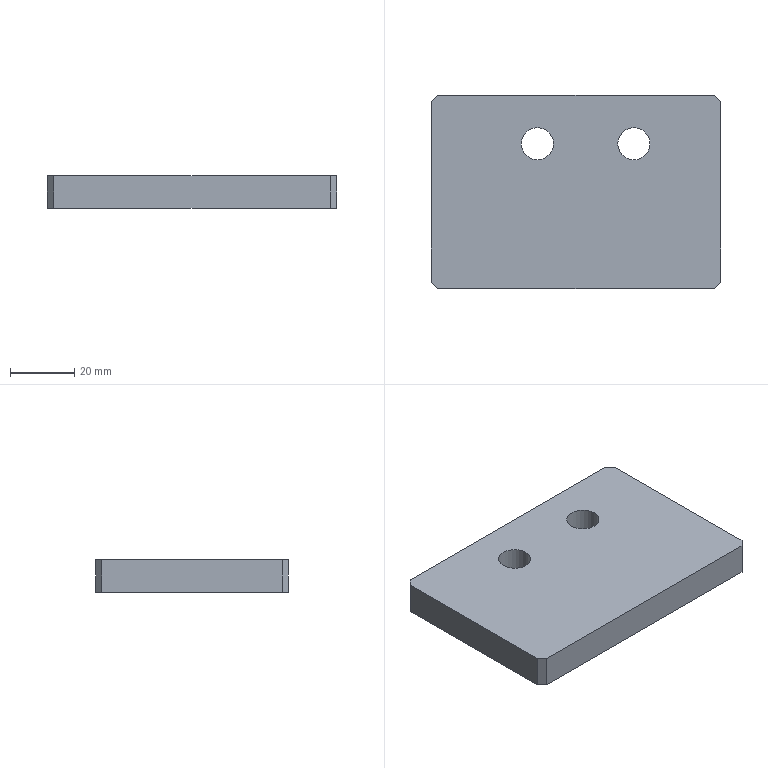Part | NX | 1 solid | 12 faces | box 90 x 60 x 10 mm | volume 52349 mm3 | plane 10 | cylinder 2 | commonest cylinder face diameters 10 x2
STEP:
#1=CARTESIAN_POINT('',(68.,45.,10.));
#2=VERTEX_POINT('',#1);
#3=CARTESIAN_POINT('',(63.,45.,10.));
#4=DIRECTION('',(0.,0.,1.));
#5=DIRECTION('',(1.,0.,0.));
#6=AXIS2_PLACEMENT_3D('',#3,#4,#5);
#7=CIRCLE('',#6,5.);
#8=EDGE_CURVE('',#2,#2,#7,.T.);
#9=ORIENTED_EDGE('',*,*,#8,.F.);
#10=EDGE_LOOP('',(#9));
#11=FACE_BOUND('',#10,.T.);
#12=CARTESIAN_POINT('',(38.,45.,10.));
#13=VERTEX_POINT('',#12);
#14=CARTESIAN_POINT('',(33.,45.,10.));
#15=DIRECTION('',(0.,0.,1.));
#16=DIRECTION('',(1.,0.,0.));
#17=AXIS2_PLACEMENT_3D('',#14,#15,#16);
#18=CIRCLE('',#17,5.);
#19=EDGE_CURVE('',#13,#13,#18,.T.);
#20=ORIENTED_EDGE('',*,*,#19,.F.);
#21=EDGE_LOOP('',(#20));
#22=FACE_BOUND('',#21,.T.);
#23=CARTESIAN_POINT('',(0.,2.,10.));
#24=VERTEX_POINT('',#23);
#25=CARTESIAN_POINT('',(0.,58.,10.));
#26=VERTEX_POINT('',#25);
#27=CARTESIAN_POINT('',(0.,30.,10.));
#28=DIRECTION('',(0.,1.,0.));
#29=VECTOR('',#28,1000.);
#30=LINE('',#27,#29);
#31=EDGE_CURVE('',#24,#26,#30,.T.);
#32=ORIENTED_EDGE('',*,*,#31,.F.);
#33=CARTESIAN_POINT('',(2.,0.,10.));
#34=VERTEX_POINT('',#33);
#35=CARTESIAN_POINT('',(8.5,-6.5,10.));
#36=DIRECTION('',(-0.7071,0.7071,0.));
#37=VECTOR('',#36,1000.);
#38=LINE('',#35,#37);
#39=EDGE_CURVE('',#24,#34,#38,.F.);
#40=ORIENTED_EDGE('',*,*,#39,.T.);
#41=CARTESIAN_POINT('',(88.,0.,10.));
#42=VERTEX_POINT('',#41);
#43=CARTESIAN_POINT('',(45.,0.,10.));
#44=DIRECTION('',(-1.,0.,0.));
#45=VECTOR('',#44,1000.);
#46=LINE('',#43,#45);
#47=EDGE_CURVE('',#42,#34,#46,.T.);
#48=ORIENTED_EDGE('',*,*,#47,.F.);
#49=CARTESIAN_POINT('',(90.,2.,10.));
#50=VERTEX_POINT('',#49);
#51=CARTESIAN_POINT('',(81.5,-6.5,10.));
#52=DIRECTION('',(-0.7071,-0.7071,0.));
#53=VECTOR('',#52,1000.);
#54=LINE('',#51,#53);
#55=EDGE_CURVE('',#42,#50,#54,.F.);
#56=ORIENTED_EDGE('',*,*,#55,.T.);
#57=CARTESIAN_POINT('',(90.,58.,10.));
#58=VERTEX_POINT('',#57);
#59=CARTESIAN_POINT('',(90.,30.,10.));
#60=DIRECTION('',(0.,-1.,0.));
#61=VECTOR('',#60,1000.);
#62=LINE('',#59,#61);
#63=EDGE_CURVE('',#58,#50,#62,.T.);
#64=ORIENTED_EDGE('',*,*,#63,.F.);
#65=CARTESIAN_POINT('',(88.,60.,10.));
#66=VERTEX_POINT('',#65);
#67=CARTESIAN_POINT('',(81.5,66.5,10.));
#68=DIRECTION('',(0.7071,-0.7071,0.));
#69=VECTOR('',#68,1000.);
#70=LINE('',#67,#69);
#71=EDGE_CURVE('',#58,#66,#70,.F.);
#72=ORIENTED_EDGE('',*,*,#71,.T.);
#73=CARTESIAN_POINT('',(2.,60.,10.));
#74=VERTEX_POINT('',#73);
#75=CARTESIAN_POINT('',(45.,60.,10.));
#76=DIRECTION('',(1.,0.,0.));
#77=VECTOR('',#76,1000.);
#78=LINE('',#75,#77);
#79=EDGE_CURVE('',#74,#66,#78,.T.);
#80=ORIENTED_EDGE('',*,*,#79,.F.);
#81=CARTESIAN_POINT('',(8.5,66.5,10.));
#82=DIRECTION('',(0.7071,0.7071,0.));
#83=VECTOR('',#82,1000.);
#84=LINE('',#81,#83);
#85=EDGE_CURVE('',#74,#26,#84,.F.);
#86=ORIENTED_EDGE('',*,*,#85,.T.);
#87=EDGE_LOOP('',(#32,#40,#48,#56,#64,#72,#80,#86));
#88=FACE_BOUND('',#87,.T.);
#89=CARTESIAN_POINT('',(45.,30.,10.));
#90=DIRECTION('',(0.,0.,1.));
#91=DIRECTION('',(1.,0.,0.));
#92=AXIS2_PLACEMENT_3D('',#89,#90,#91);
#93=PLANE('',#92);
#94=ADVANCED_FACE('',(#11,#22,#88),#93,.T.);
#95=ORIENTED_EDGE('',*,*,#47,.T.);
#96=CARTESIAN_POINT('',(2.,0.,0.));
#97=VERTEX_POINT('',#96);
#98=CARTESIAN_POINT('',(2.,0.,0.));
#99=DIRECTION('',(0.,0.,-1.));
#100=VECTOR('',#99,1000.);
#101=LINE('',#98,#100);
#102=EDGE_CURVE('',#34,#97,#101,.T.);
#103=ORIENTED_EDGE('',*,*,#102,.T.);
#104=CARTESIAN_POINT('',(88.,0.,0.));
#105=VERTEX_POINT('',#104);
#106=CARTESIAN_POINT('',(45.,0.,0.));
#107=DIRECTION('',(1.,0.,0.));
#108=VECTOR('',#107,1000.);
#109=LINE('',#106,#108);
#110=EDGE_CURVE('',#97,#105,#109,.T.);
#111=ORIENTED_EDGE('',*,*,#110,.T.);
#112=CARTESIAN_POINT('',(88.,0.,0.));
#113=DIRECTION('',(0.,0.,1.));
#114=VECTOR('',#113,1000.);
#115=LINE('',#112,#114);
#116=EDGE_CURVE('',#105,#42,#115,.T.);
#117=ORIENTED_EDGE('',*,*,#116,.T.);
#118=EDGE_LOOP('',(#95,#103,#111,#117));
#119=FACE_BOUND('',#118,.T.);
#120=CARTESIAN_POINT('',(45.,0.,0.));
#121=DIRECTION('',(0.,-1.,0.));
#122=DIRECTION('',(0.,0.,-1.));
#123=AXIS2_PLACEMENT_3D('',#120,#121,#122);
#124=PLANE('',#123);
#125=ADVANCED_FACE('',(#119),#124,.T.);
#126=CARTESIAN_POINT('',(0.,58.,0.));
#127=VERTEX_POINT('',#126);
#128=CARTESIAN_POINT('',(0.,2.,0.));
#129=VERTEX_POINT('',#128);
#130=CARTESIAN_POINT('',(0.,30.,0.));
#131=DIRECTION('',(0.,-1.,0.));
#132=VECTOR('',#131,1000.);
#133=LINE('',#130,#132);
#134=EDGE_CURVE('',#127,#129,#133,.T.);
#135=ORIENTED_EDGE('',*,*,#134,.T.);
#136=CARTESIAN_POINT('',(0.,2.,0.));
#137=DIRECTION('',(0.,0.,1.));
#138=VECTOR('',#137,1000.);
#139=LINE('',#136,#138);
#140=EDGE_CURVE('',#129,#24,#139,.T.);
#141=ORIENTED_EDGE('',*,*,#140,.T.);
#142=ORIENTED_EDGE('',*,*,#31,.T.);
#143=CARTESIAN_POINT('',(0.,58.,0.));
#144=DIRECTION('',(0.,0.,-1.));
#145=VECTOR('',#144,1000.);
#146=LINE('',#143,#145);
#147=EDGE_CURVE('',#26,#127,#146,.T.);
#148=ORIENTED_EDGE('',*,*,#147,.T.);
#149=EDGE_LOOP('',(#135,#141,#142,#148));
#150=FACE_BOUND('',#149,.T.);
#151=CARTESIAN_POINT('',(0.,30.,0.));
#152=DIRECTION('',(-1.,0.,0.));
#153=DIRECTION('',(0.,0.,1.));
#154=AXIS2_PLACEMENT_3D('',#151,#152,#153);
#155=PLANE('',#154);
#156=ADVANCED_FACE('',(#150),#155,.T.);
#157=ORIENTED_EDGE('',*,*,#79,.T.);
#158=CARTESIAN_POINT('',(88.,60.,0.));
#159=VERTEX_POINT('',#158);
#160=CARTESIAN_POINT('',(88.,60.,0.));
#161=DIRECTION('',(0.,0.,-1.));
#162=VECTOR('',#161,1000.);
#163=LINE('',#160,#162);
#164=EDGE_CURVE('',#66,#159,#163,.T.);
#165=ORIENTED_EDGE('',*,*,#164,.T.);
#166=CARTESIAN_POINT('',(2.,60.,0.));
#167=VERTEX_POINT('',#166);
#168=CARTESIAN_POINT('',(45.,60.,0.));
#169=DIRECTION('',(-1.,0.,0.));
#170=VECTOR('',#169,1000.);
#171=LINE('',#168,#170);
#172=EDGE_CURVE('',#159,#167,#171,.T.);
#173=ORIENTED_EDGE('',*,*,#172,.T.);
#174=CARTESIAN_POINT('',(2.,60.,0.));
#175=DIRECTION('',(0.,0.,1.));
#176=VECTOR('',#175,1000.);
#177=LINE('',#174,#176);
#178=EDGE_CURVE('',#167,#74,#177,.T.);
#179=ORIENTED_EDGE('',*,*,#178,.T.);
#180=EDGE_LOOP('',(#157,#165,#173,#179));
#181=FACE_BOUND('',#180,.T.);
#182=CARTESIAN_POINT('',(45.,60.,0.));
#183=DIRECTION('',(0.,1.,0.));
#184=DIRECTION('',(0.,0.,1.));
#185=AXIS2_PLACEMENT_3D('',#182,#183,#184);
#186=PLANE('',#185);
#187=ADVANCED_FACE('',(#181),#186,.T.);
#188=CARTESIAN_POINT('',(68.,45.,0.));
#189=VERTEX_POINT('',#188);
#190=CARTESIAN_POINT('',(63.,45.,0.));
#191=DIRECTION('',(0.,0.,1.));
#192=DIRECTION('',(1.,0.,0.));
#193=AXIS2_PLACEMENT_3D('',#190,#191,#192);
#194=CIRCLE('',#193,5.);
#195=EDGE_CURVE('',#189,#189,#194,.T.);
#196=ORIENTED_EDGE('',*,*,#195,.T.);
#197=EDGE_LOOP('',(#196));
#198=FACE_BOUND('',#197,.T.);
#199=CARTESIAN_POINT('',(38.,45.,0.));
#200=VERTEX_POINT('',#199);
#201=CARTESIAN_POINT('',(33.,45.,0.));
#202=DIRECTION('',(0.,0.,1.));
#203=DIRECTION('',(1.,0.,0.));
#204=AXIS2_PLACEMENT_3D('',#201,#202,#203);
#205=CIRCLE('',#204,5.);
#206=EDGE_CURVE('',#200,#200,#205,.T.);
#207=ORIENTED_EDGE('',*,*,#206,.T.);
#208=EDGE_LOOP('',(#207));
#209=FACE_BOUND('',#208,.T.);
#210=ORIENTED_EDGE('',*,*,#110,.F.);
#211=CARTESIAN_POINT('',(8.5,-6.5,0.));
#212=DIRECTION('',(0.7071,-0.7071,0.));
#213=VECTOR('',#212,1000.);
#214=LINE('',#211,#213);
#215=EDGE_CURVE('',#97,#129,#214,.F.);
#216=ORIENTED_EDGE('',*,*,#215,.T.);
#217=ORIENTED_EDGE('',*,*,#134,.F.);
#218=CARTESIAN_POINT('',(8.5,66.5,0.));
#219=DIRECTION('',(-0.7071,-0.7071,0.));
#220=VECTOR('',#219,1000.);
#221=LINE('',#218,#220);
#222=EDGE_CURVE('',#127,#167,#221,.F.);
#223=ORIENTED_EDGE('',*,*,#222,.T.);
#224=ORIENTED_EDGE('',*,*,#172,.F.);
#225=CARTESIAN_POINT('',(90.,58.,0.));
#226=VERTEX_POINT('',#225);
#227=CARTESIAN_POINT('',(81.5,66.5,0.));
#228=DIRECTION('',(-0.7071,0.7071,0.));
#229=VECTOR('',#228,1000.);
#230=LINE('',#227,#229);
#231=EDGE_CURVE('',#159,#226,#230,.F.);
#232=ORIENTED_EDGE('',*,*,#231,.T.);
#233=CARTESIAN_POINT('',(90.,2.,0.));
#234=VERTEX_POINT('',#233);
#235=CARTESIAN_POINT('',(90.,30.,0.));
#236=DIRECTION('',(0.,1.,0.));
#237=VECTOR('',#236,1000.);
#238=LINE('',#235,#237);
#239=EDGE_CURVE('',#234,#226,#238,.T.);
#240=ORIENTED_EDGE('',*,*,#239,.F.);
#241=CARTESIAN_POINT('',(81.5,-6.5,0.));
#242=DIRECTION('',(0.7071,0.7071,0.));
#243=VECTOR('',#242,1000.);
#244=LINE('',#241,#243);
#245=EDGE_CURVE('',#234,#105,#244,.F.);
#246=ORIENTED_EDGE('',*,*,#245,.T.);
#247=EDGE_LOOP('',(#210,#216,#217,#223,#224,#232,#240,#246));
#248=FACE_BOUND('',#247,.T.);
#249=CARTESIAN_POINT('',(45.,30.,0.));
#250=DIRECTION('',(0.,0.,-1.));
#251=DIRECTION('',(-1.,0.,0.));
#252=AXIS2_PLACEMENT_3D('',#249,#250,#251);
#253=PLANE('',#252);
#254=ADVANCED_FACE('',(#198,#209,#248),#253,.T.);
#255=ORIENTED_EDGE('',*,*,#63,.T.);
#256=CARTESIAN_POINT('',(90.,2.,0.));
#257=DIRECTION('',(0.,0.,-1.));
#258=VECTOR('',#257,1000.);
#259=LINE('',#256,#258);
#260=EDGE_CURVE('',#50,#234,#259,.T.);
#261=ORIENTED_EDGE('',*,*,#260,.T.);
#262=ORIENTED_EDGE('',*,*,#239,.T.);
#263=CARTESIAN_POINT('',(90.,58.,0.));
#264=DIRECTION('',(0.,0.,1.));
#265=VECTOR('',#264,1000.);
#266=LINE('',#263,#265);
#267=EDGE_CURVE('',#226,#58,#266,.T.);
#268=ORIENTED_EDGE('',*,*,#267,.T.);
#269=EDGE_LOOP('',(#255,#261,#262,#268));
#270=FACE_BOUND('',#269,.T.);
#271=CARTESIAN_POINT('',(90.,30.,0.));
#272=DIRECTION('',(1.,0.,0.));
#273=DIRECTION('',(0.,0.,-1.));
#274=AXIS2_PLACEMENT_3D('',#271,#272,#273);
#275=PLANE('',#274);
#276=ADVANCED_FACE('',(#270),#275,.T.);
#277=ORIENTED_EDGE('',*,*,#19,.T.);
#278=EDGE_LOOP('',(#277));
#279=FACE_BOUND('',#278,.T.);
#280=ORIENTED_EDGE('',*,*,#206,.F.);
#281=EDGE_LOOP('',(#280));
#282=FACE_BOUND('',#281,.T.);
#283=CARTESIAN_POINT('',(33.,45.,0.));
#284=DIRECTION('',(0.,0.,1.));
#285=DIRECTION('',(1.,0.,0.));
#286=AXIS2_PLACEMENT_3D('',#283,#284,#285);
#287=CYLINDRICAL_SURFACE('',#286,5.);
#288=ADVANCED_FACE('',(#279,#282),#287,.F.);
#289=ORIENTED_EDGE('',*,*,#8,.T.);
#290=EDGE_LOOP('',(#289));
#291=FACE_BOUND('',#290,.T.);
#292=ORIENTED_EDGE('',*,*,#195,.F.);
#293=EDGE_LOOP('',(#292));
#294=FACE_BOUND('',#293,.T.);
#295=CARTESIAN_POINT('',(63.,45.,0.));
#296=DIRECTION('',(0.,0.,1.));
#297=DIRECTION('',(1.,0.,0.));
#298=AXIS2_PLACEMENT_3D('',#295,#296,#297);
#299=CYLINDRICAL_SURFACE('',#298,5.);
#300=ADVANCED_FACE('',(#291,#294),#299,.F.);
#301=ORIENTED_EDGE('',*,*,#215,.F.);
#302=ORIENTED_EDGE('',*,*,#102,.F.);
#303=ORIENTED_EDGE('',*,*,#39,.F.);
#304=ORIENTED_EDGE('',*,*,#140,.F.);
#305=EDGE_LOOP('',(#301,#302,#303,#304));
#306=FACE_BOUND('',#305,.T.);
#307=CARTESIAN_POINT('',(0.,2.,0.));
#308=DIRECTION('',(0.7071,0.7071,0.));
#309=DIRECTION('',(0.,0.,1.));
#310=AXIS2_PLACEMENT_3D('',#307,#308,#309);
#311=PLANE('',#310);
#312=ADVANCED_FACE('',(#306),#311,.F.);
#313=ORIENTED_EDGE('',*,*,#245,.F.);
#314=ORIENTED_EDGE('',*,*,#260,.F.);
#315=ORIENTED_EDGE('',*,*,#55,.F.);
#316=ORIENTED_EDGE('',*,*,#116,.F.);
#317=EDGE_LOOP('',(#313,#314,#315,#316));
#318=FACE_BOUND('',#317,.T.);
#319=CARTESIAN_POINT('',(88.,0.,0.));
#320=DIRECTION('',(-0.7071,0.7071,0.));
#321=DIRECTION('',(0.,0.,1.));
#322=AXIS2_PLACEMENT_3D('',#319,#320,#321);
#323=PLANE('',#322);
#324=ADVANCED_FACE('',(#318),#323,.F.);
#325=ORIENTED_EDGE('',*,*,#231,.F.);
#326=ORIENTED_EDGE('',*,*,#164,.F.);
#327=ORIENTED_EDGE('',*,*,#71,.F.);
#328=ORIENTED_EDGE('',*,*,#267,.F.);
#329=EDGE_LOOP('',(#325,#326,#327,#328));
#330=FACE_BOUND('',#329,.T.);
#331=CARTESIAN_POINT('',(90.,58.,0.));
#332=DIRECTION('',(-0.7071,-0.7071,0.));
#333=DIRECTION('',(0.,0.,1.));
#334=AXIS2_PLACEMENT_3D('',#331,#332,#333);
#335=PLANE('',#334);
#336=ADVANCED_FACE('',(#330),#335,.F.);
#337=ORIENTED_EDGE('',*,*,#222,.F.);
#338=ORIENTED_EDGE('',*,*,#147,.F.);
#339=ORIENTED_EDGE('',*,*,#85,.F.);
#340=ORIENTED_EDGE('',*,*,#178,.F.);
#341=EDGE_LOOP('',(#337,#338,#339,#340));
#342=FACE_BOUND('',#341,.T.);
#343=CARTESIAN_POINT('',(2.,60.,0.));
#344=DIRECTION('',(0.7071,-0.7071,0.));
#345=DIRECTION('',(0.,0.,1.));
#346=AXIS2_PLACEMENT_3D('',#343,#344,#345);
#347=PLANE('',#346);
#348=ADVANCED_FACE('',(#342),#347,.F.);
#349=CLOSED_SHELL('',(#94,#125,#156,#187,#254,#276,#288,#300,#312,#324,#336,#348));
#350=MANIFOLD_SOLID_BREP('',#349);
#351=(LENGTH_UNIT()NAMED_UNIT(*)SI_UNIT(.MILLI.,.METRE.));
#352=UNCERTAINTY_MEASURE_WITH_UNIT(LENGTH_MEASURE(0.00001),#351,'','');
#353=(NAMED_UNIT(*)PLANE_ANGLE_UNIT()SI_UNIT($,.RADIAN.));
#354=(NAMED_UNIT(*)SI_UNIT($,.STERADIAN.)SOLID_ANGLE_UNIT());
#355=(GEOMETRIC_REPRESENTATION_CONTEXT(3)GLOBAL_UNCERTAINTY_ASSIGNED_CONTEXT((#352))GLOBAL_UNIT_ASSIGNED_CONTEXT((#351,#353,#354))REPRESENTATION_CONTEXT('',''));
#356=ADVANCED_BREP_SHAPE_REPRESENTATION('',(#350),#355);